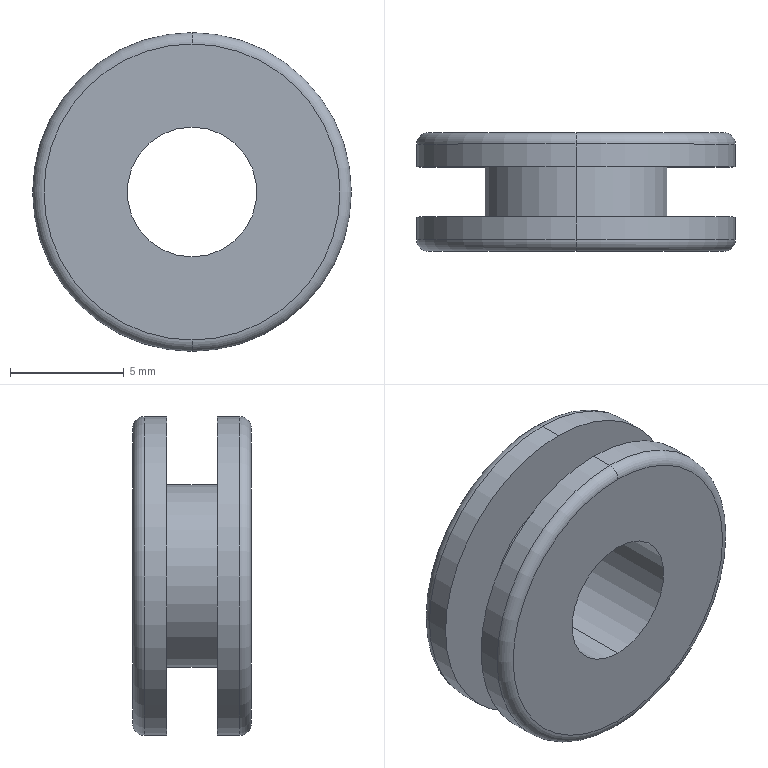Part | SolidWorks | features Revolution 1 | 1 solid | 16 faces | box 14 x 5.2 x 14 mm | volume 435.063 mm3 | cylinder 8 | torus 4 | plane 4 | commonest cylinder face diameters 14 x4 5.7 x2 8 x2
STEP:
#1=CARTESIAN_POINT('',(0.,0.5,-7.));
#2=VERTEX_POINT('',#1);
#3=CARTESIAN_POINT('',(0.,0.5,7.));
#4=VERTEX_POINT('',#3);
#5=CARTESIAN_POINT('',(0.,0.5,0.));
#6=DIRECTION('',(0.,-1.,0.));
#7=DIRECTION('',(0.,0.,-1.));
#8=AXIS2_PLACEMENT_3D('',#5,#6,#7);
#9=CIRCLE('',#8,7.);
#10=EDGE_CURVE('',#2,#4,#9,.T.);
#11=ORIENTED_EDGE('',*,*,#10,.T.);
#12=CARTESIAN_POINT('',(0.,0.,6.5));
#13=VERTEX_POINT('',#12);
#14=CARTESIAN_POINT('',(0.,0.5,6.5));
#15=DIRECTION('',(1.,0.,0.));
#16=DIRECTION('',(0.,0.,-1.));
#17=AXIS2_PLACEMENT_3D('',#14,#15,#16);
#18=CIRCLE('',#17,0.5);
#19=EDGE_CURVE('',#4,#13,#18,.T.);
#20=ORIENTED_EDGE('',*,*,#19,.T.);
#21=CARTESIAN_POINT('',(0.,0.,-6.5));
#22=VERTEX_POINT('',#21);
#23=CARTESIAN_POINT('',(0.,0.,0.));
#24=DIRECTION('',(0.,-1.,0.));
#25=DIRECTION('',(0.,0.,-1.));
#26=AXIS2_PLACEMENT_3D('',#23,#24,#25);
#27=CIRCLE('',#26,6.5);
#28=EDGE_CURVE('',#22,#13,#27,.T.);
#29=ORIENTED_EDGE('',*,*,#28,.F.);
#30=CARTESIAN_POINT('',(0.,0.5,-6.5));
#31=DIRECTION('',(-1.,0.,0.));
#32=DIRECTION('',(0.,0.,1.));
#33=AXIS2_PLACEMENT_3D('',#30,#31,#32);
#34=CIRCLE('',#33,0.5);
#35=EDGE_CURVE('',#2,#22,#34,.T.);
#36=ORIENTED_EDGE('',*,*,#35,.F.);
#37=EDGE_LOOP('',(#11,#20,#29,#36));
#38=FACE_OUTER_BOUND('',#37,.T.);
#39=CARTESIAN_POINT('',(0.,0.5,0.));
#40=DIRECTION('',(0.,-1.,0.));
#41=DIRECTION('',(0.,0.,-1.));
#42=AXIS2_PLACEMENT_3D('',#39,#40,#41);
#43=TOROIDAL_SURFACE('',#42,6.5,0.5);
#44=ADVANCED_FACE('',(#38),#43,.T.);
#45=CARTESIAN_POINT('',(0.,1.5,-7.));
#46=VERTEX_POINT('',#45);
#47=CARTESIAN_POINT('',(0.,1.5,7.));
#48=VERTEX_POINT('',#47);
#49=CARTESIAN_POINT('',(0.,1.5,0.));
#50=DIRECTION('',(0.,-1.,0.));
#51=DIRECTION('',(0.,0.,-1.));
#52=AXIS2_PLACEMENT_3D('',#49,#50,#51);
#53=CIRCLE('',#52,7.);
#54=EDGE_CURVE('',#46,#48,#53,.T.);
#55=ORIENTED_EDGE('',*,*,#54,.T.);
#56=CARTESIAN_POINT('',(0.,0.,7.));
#57=DIRECTION('',(0.,-1.,0.));
#58=VECTOR('',#57,1000.);
#59=LINE('',#56,#58);
#60=EDGE_CURVE('',#48,#4,#59,.T.);
#61=ORIENTED_EDGE('',*,*,#60,.T.);
#62=ORIENTED_EDGE('',*,*,#10,.F.);
#63=CARTESIAN_POINT('',(0.,0.,-7.));
#64=DIRECTION('',(0.,-1.,0.));
#65=VECTOR('',#64,1000.);
#66=LINE('',#63,#65);
#67=EDGE_CURVE('',#46,#2,#66,.T.);
#68=ORIENTED_EDGE('',*,*,#67,.F.);
#69=EDGE_LOOP('',(#55,#61,#62,#68));
#70=FACE_OUTER_BOUND('',#69,.T.);
#71=CARTESIAN_POINT('',(0.,0.,0.));
#72=DIRECTION('',(0.,-1.,0.));
#73=DIRECTION('',(0.,0.,-1.));
#74=AXIS2_PLACEMENT_3D('',#71,#72,#73);
#75=CYLINDRICAL_SURFACE('',#74,7.);
#76=ADVANCED_FACE('',(#70),#75,.T.);
#77=CARTESIAN_POINT('',(0.,3.7,-4.));
#78=VERTEX_POINT('',#77);
#79=CARTESIAN_POINT('',(0.,3.7,4.));
#80=VERTEX_POINT('',#79);
#81=CARTESIAN_POINT('',(0.,3.7,0.));
#82=DIRECTION('',(0.,-1.,0.));
#83=DIRECTION('',(0.,0.,-1.));
#84=AXIS2_PLACEMENT_3D('',#81,#82,#83);
#85=CIRCLE('',#84,4.);
#86=EDGE_CURVE('',#78,#80,#85,.T.);
#87=ORIENTED_EDGE('',*,*,#86,.T.);
#88=CARTESIAN_POINT('',(0.,1.5,4.));
#89=VERTEX_POINT('',#88);
#90=CARTESIAN_POINT('',(0.,0.,4.));
#91=DIRECTION('',(0.,-1.,0.));
#92=VECTOR('',#91,1000.);
#93=LINE('',#90,#92);
#94=EDGE_CURVE('',#80,#89,#93,.T.);
#95=ORIENTED_EDGE('',*,*,#94,.T.);
#96=CARTESIAN_POINT('',(0.,1.5,-4.));
#97=VERTEX_POINT('',#96);
#98=CARTESIAN_POINT('',(0.,1.5,0.));
#99=DIRECTION('',(0.,-1.,0.));
#100=DIRECTION('',(0.,0.,-1.));
#101=AXIS2_PLACEMENT_3D('',#98,#99,#100);
#102=CIRCLE('',#101,4.);
#103=EDGE_CURVE('',#97,#89,#102,.T.);
#104=ORIENTED_EDGE('',*,*,#103,.F.);
#105=CARTESIAN_POINT('',(0.,0.,-4.));
#106=DIRECTION('',(0.,-1.,0.));
#107=VECTOR('',#106,1000.);
#108=LINE('',#105,#107);
#109=EDGE_CURVE('',#78,#97,#108,.T.);
#110=ORIENTED_EDGE('',*,*,#109,.F.);
#111=EDGE_LOOP('',(#87,#95,#104,#110));
#112=FACE_OUTER_BOUND('',#111,.T.);
#113=CARTESIAN_POINT('',(0.,0.,0.));
#114=DIRECTION('',(0.,-1.,0.));
#115=DIRECTION('',(0.,0.,-1.));
#116=AXIS2_PLACEMENT_3D('',#113,#114,#115);
#117=CYLINDRICAL_SURFACE('',#116,4.);
#118=ADVANCED_FACE('',(#112),#117,.T.);
#119=CARTESIAN_POINT('',(0.,4.7,-7.));
#120=VERTEX_POINT('',#119);
#121=CARTESIAN_POINT('',(0.,4.7,7.));
#122=VERTEX_POINT('',#121);
#123=CARTESIAN_POINT('',(0.,4.7,0.));
#124=DIRECTION('',(0.,-1.,0.));
#125=DIRECTION('',(0.,0.,-1.));
#126=AXIS2_PLACEMENT_3D('',#123,#124,#125);
#127=CIRCLE('',#126,7.);
#128=EDGE_CURVE('',#120,#122,#127,.T.);
#129=ORIENTED_EDGE('',*,*,#128,.T.);
#130=CARTESIAN_POINT('',(0.,3.7,7.));
#131=VERTEX_POINT('',#130);
#132=CARTESIAN_POINT('',(0.,0.,7.));
#133=DIRECTION('',(0.,-1.,0.));
#134=VECTOR('',#133,1000.);
#135=LINE('',#132,#134);
#136=EDGE_CURVE('',#122,#131,#135,.T.);
#137=ORIENTED_EDGE('',*,*,#136,.T.);
#138=CARTESIAN_POINT('',(0.,3.7,-7.));
#139=VERTEX_POINT('',#138);
#140=CARTESIAN_POINT('',(0.,3.7,0.));
#141=DIRECTION('',(0.,-1.,0.));
#142=DIRECTION('',(0.,0.,-1.));
#143=AXIS2_PLACEMENT_3D('',#140,#141,#142);
#144=CIRCLE('',#143,7.);
#145=EDGE_CURVE('',#139,#131,#144,.T.);
#146=ORIENTED_EDGE('',*,*,#145,.F.);
#147=CARTESIAN_POINT('',(0.,0.,-7.));
#148=DIRECTION('',(0.,-1.,0.));
#149=VECTOR('',#148,1000.);
#150=LINE('',#147,#149);
#151=EDGE_CURVE('',#120,#139,#150,.T.);
#152=ORIENTED_EDGE('',*,*,#151,.F.);
#153=EDGE_LOOP('',(#129,#137,#146,#152));
#154=FACE_OUTER_BOUND('',#153,.T.);
#155=CARTESIAN_POINT('',(0.,0.,0.));
#156=DIRECTION('',(0.,-1.,0.));
#157=DIRECTION('',(0.,0.,-1.));
#158=AXIS2_PLACEMENT_3D('',#155,#156,#157);
#159=CYLINDRICAL_SURFACE('',#158,7.);
#160=ADVANCED_FACE('',(#154),#159,.T.);
#161=CARTESIAN_POINT('',(0.,5.2,-6.5));
#162=VERTEX_POINT('',#161);
#163=CARTESIAN_POINT('',(0.,5.2,6.5));
#164=VERTEX_POINT('',#163);
#165=CARTESIAN_POINT('',(0.,5.2,0.));
#166=DIRECTION('',(0.,-1.,0.));
#167=DIRECTION('',(0.,0.,-1.));
#168=AXIS2_PLACEMENT_3D('',#165,#166,#167);
#169=CIRCLE('',#168,6.5);
#170=EDGE_CURVE('',#162,#164,#169,.T.);
#171=ORIENTED_EDGE('',*,*,#170,.T.);
#172=CARTESIAN_POINT('',(0.,4.7,6.5));
#173=DIRECTION('',(1.,0.,0.));
#174=DIRECTION('',(0.,0.,-1.));
#175=AXIS2_PLACEMENT_3D('',#172,#173,#174);
#176=CIRCLE('',#175,0.5);
#177=EDGE_CURVE('',#164,#122,#176,.T.);
#178=ORIENTED_EDGE('',*,*,#177,.T.);
#179=ORIENTED_EDGE('',*,*,#128,.F.);
#180=CARTESIAN_POINT('',(0.,4.7,-6.5));
#181=DIRECTION('',(-1.,0.,0.));
#182=DIRECTION('',(0.,0.,1.));
#183=AXIS2_PLACEMENT_3D('',#180,#181,#182);
#184=CIRCLE('',#183,0.5);
#185=EDGE_CURVE('',#162,#120,#184,.T.);
#186=ORIENTED_EDGE('',*,*,#185,.F.);
#187=EDGE_LOOP('',(#171,#178,#179,#186));
#188=FACE_OUTER_BOUND('',#187,.T.);
#189=CARTESIAN_POINT('',(0.,4.7,0.));
#190=DIRECTION('',(0.,-1.,0.));
#191=DIRECTION('',(0.,0.,-1.));
#192=AXIS2_PLACEMENT_3D('',#189,#190,#191);
#193=TOROIDAL_SURFACE('',#192,6.5,0.5);
#194=ADVANCED_FACE('',(#188),#193,.T.);
#195=CARTESIAN_POINT('',(0.,5.2,2.85));
#196=VERTEX_POINT('',#195);
#197=CARTESIAN_POINT('',(0.,5.2,-2.85));
#198=VERTEX_POINT('',#197);
#199=CARTESIAN_POINT('',(0.,5.2,0.));
#200=DIRECTION('',(0.,-1.,0.));
#201=DIRECTION('',(0.,0.,-1.));
#202=AXIS2_PLACEMENT_3D('',#199,#200,#201);
#203=CIRCLE('',#202,2.85);
#204=EDGE_CURVE('',#196,#198,#203,.T.);
#205=ORIENTED_EDGE('',*,*,#204,.F.);
#206=CARTESIAN_POINT('',(0.,0.,2.85));
#207=VERTEX_POINT('',#206);
#208=CARTESIAN_POINT('',(0.,0.,2.85));
#209=DIRECTION('',(0.,-1.,0.));
#210=VECTOR('',#209,1000.);
#211=LINE('',#208,#210);
#212=EDGE_CURVE('',#196,#207,#211,.T.);
#213=ORIENTED_EDGE('',*,*,#212,.T.);
#214=CARTESIAN_POINT('',(0.,0.,-2.85));
#215=VERTEX_POINT('',#214);
#216=CARTESIAN_POINT('',(0.,0.,0.));
#217=DIRECTION('',(0.,-1.,0.));
#218=DIRECTION('',(0.,0.,-1.));
#219=AXIS2_PLACEMENT_3D('',#216,#217,#218);
#220=CIRCLE('',#219,2.85);
#221=EDGE_CURVE('',#207,#215,#220,.T.);
#222=ORIENTED_EDGE('',*,*,#221,.T.);
#223=CARTESIAN_POINT('',(0.,0.,-2.85));
#224=DIRECTION('',(0.,-1.,0.));
#225=VECTOR('',#224,1000.);
#226=LINE('',#223,#225);
#227=EDGE_CURVE('',#198,#215,#226,.T.);
#228=ORIENTED_EDGE('',*,*,#227,.F.);
#229=EDGE_LOOP('',(#205,#213,#222,#228));
#230=FACE_OUTER_BOUND('',#229,.T.);
#231=CARTESIAN_POINT('',(0.,0.,0.));
#232=DIRECTION('',(0.,-1.,0.));
#233=DIRECTION('',(0.,0.,-1.));
#234=AXIS2_PLACEMENT_3D('',#231,#232,#233);
#235=CYLINDRICAL_SURFACE('',#234,2.85);
#236=ADVANCED_FACE('',(#230),#235,.F.);
#237=ORIENTED_EDGE('',*,*,#212,.F.);
#238=CARTESIAN_POINT('',(0.,5.2,0.));
#239=DIRECTION('',(0.,-1.,0.));
#240=DIRECTION('',(0.,0.,-1.));
#241=AXIS2_PLACEMENT_3D('',#238,#239,#240);
#242=CIRCLE('',#241,2.85);
#243=EDGE_CURVE('',#198,#196,#242,.T.);
#244=ORIENTED_EDGE('',*,*,#243,.F.);
#245=ORIENTED_EDGE('',*,*,#227,.T.);
#246=CARTESIAN_POINT('',(0.,0.,0.));
#247=DIRECTION('',(0.,-1.,0.));
#248=DIRECTION('',(0.,0.,-1.));
#249=AXIS2_PLACEMENT_3D('',#246,#247,#248);
#250=CIRCLE('',#249,2.85);
#251=EDGE_CURVE('',#215,#207,#250,.T.);
#252=ORIENTED_EDGE('',*,*,#251,.T.);
#253=EDGE_LOOP('',(#237,#244,#245,#252));
#254=FACE_OUTER_BOUND('',#253,.T.);
#255=CARTESIAN_POINT('',(0.,0.,0.));
#256=DIRECTION('',(0.,-1.,0.));
#257=DIRECTION('',(0.,0.,-1.));
#258=AXIS2_PLACEMENT_3D('',#255,#256,#257);
#259=CYLINDRICAL_SURFACE('',#258,2.85);
#260=ADVANCED_FACE('',(#254),#259,.F.);
#261=ORIENTED_EDGE('',*,*,#243,.T.);
#262=ORIENTED_EDGE('',*,*,#204,.T.);
#263=EDGE_LOOP('',(#261,#262));
#264=FACE_BOUND('',#263,.T.);
#265=ORIENTED_EDGE('',*,*,#170,.F.);
#266=CARTESIAN_POINT('',(0.,5.2,0.));
#267=DIRECTION('',(0.,-1.,0.));
#268=DIRECTION('',(0.,0.,-1.));
#269=AXIS2_PLACEMENT_3D('',#266,#267,#268);
#270=CIRCLE('',#269,6.5);
#271=EDGE_CURVE('',#164,#162,#270,.T.);
#272=ORIENTED_EDGE('',*,*,#271,.F.);
#273=EDGE_LOOP('',(#265,#272));
#274=FACE_OUTER_BOUND('',#273,.T.);
#275=CARTESIAN_POINT('',(2.85,5.2,0.));
#276=DIRECTION('',(0.,1.,0.));
#277=DIRECTION('',(0.,0.,1.));
#278=AXIS2_PLACEMENT_3D('',#275,#276,#277);
#279=PLANE('',#278);
#280=ADVANCED_FACE('',(#264,#274),#279,.T.);
#281=ORIENTED_EDGE('',*,*,#177,.F.);
#282=ORIENTED_EDGE('',*,*,#271,.T.);
#283=ORIENTED_EDGE('',*,*,#185,.T.);
#284=CARTESIAN_POINT('',(0.,4.7,0.));
#285=DIRECTION('',(0.,-1.,0.));
#286=DIRECTION('',(0.,0.,-1.));
#287=AXIS2_PLACEMENT_3D('',#284,#285,#286);
#288=CIRCLE('',#287,7.);
#289=EDGE_CURVE('',#122,#120,#288,.T.);
#290=ORIENTED_EDGE('',*,*,#289,.F.);
#291=EDGE_LOOP('',(#281,#282,#283,#290));
#292=FACE_OUTER_BOUND('',#291,.T.);
#293=CARTESIAN_POINT('',(0.,4.7,0.));
#294=DIRECTION('',(0.,-1.,0.));
#295=DIRECTION('',(0.,0.,-1.));
#296=AXIS2_PLACEMENT_3D('',#293,#294,#295);
#297=TOROIDAL_SURFACE('',#296,6.5,0.5);
#298=ADVANCED_FACE('',(#292),#297,.T.);
#299=ORIENTED_EDGE('',*,*,#136,.F.);
#300=ORIENTED_EDGE('',*,*,#289,.T.);
#301=ORIENTED_EDGE('',*,*,#151,.T.);
#302=CARTESIAN_POINT('',(0.,3.7,0.));
#303=DIRECTION('',(0.,-1.,0.));
#304=DIRECTION('',(0.,0.,-1.));
#305=AXIS2_PLACEMENT_3D('',#302,#303,#304);
#306=CIRCLE('',#305,7.);
#307=EDGE_CURVE('',#131,#139,#306,.T.);
#308=ORIENTED_EDGE('',*,*,#307,.F.);
#309=EDGE_LOOP('',(#299,#300,#301,#308));
#310=FACE_OUTER_BOUND('',#309,.T.);
#311=CARTESIAN_POINT('',(0.,0.,0.));
#312=DIRECTION('',(0.,-1.,0.));
#313=DIRECTION('',(0.,0.,-1.));
#314=AXIS2_PLACEMENT_3D('',#311,#312,#313);
#315=CYLINDRICAL_SURFACE('',#314,7.);
#316=ADVANCED_FACE('',(#310),#315,.T.);
#317=ORIENTED_EDGE('',*,*,#145,.T.);
#318=ORIENTED_EDGE('',*,*,#307,.T.);
#319=EDGE_LOOP('',(#317,#318));
#320=FACE_OUTER_BOUND('',#319,.T.);
#321=ORIENTED_EDGE('',*,*,#86,.F.);
#322=CARTESIAN_POINT('',(0.,3.7,0.));
#323=DIRECTION('',(0.,-1.,0.));
#324=DIRECTION('',(0.,0.,-1.));
#325=AXIS2_PLACEMENT_3D('',#322,#323,#324);
#326=CIRCLE('',#325,4.);
#327=EDGE_CURVE('',#80,#78,#326,.T.);
#328=ORIENTED_EDGE('',*,*,#327,.F.);
#329=EDGE_LOOP('',(#321,#328));
#330=FACE_BOUND('',#329,.T.);
#331=CARTESIAN_POINT('',(7.,3.7,0.));
#332=DIRECTION('',(0.,-1.,0.));
#333=DIRECTION('',(0.,0.,-1.));
#334=AXIS2_PLACEMENT_3D('',#331,#332,#333);
#335=PLANE('',#334);
#336=ADVANCED_FACE('',(#320,#330),#335,.T.);
#337=ORIENTED_EDGE('',*,*,#94,.F.);
#338=ORIENTED_EDGE('',*,*,#327,.T.);
#339=ORIENTED_EDGE('',*,*,#109,.T.);
#340=CARTESIAN_POINT('',(0.,1.5,0.));
#341=DIRECTION('',(0.,-1.,0.));
#342=DIRECTION('',(0.,0.,-1.));
#343=AXIS2_PLACEMENT_3D('',#340,#341,#342);
#344=CIRCLE('',#343,4.);
#345=EDGE_CURVE('',#89,#97,#344,.T.);
#346=ORIENTED_EDGE('',*,*,#345,.F.);
#347=EDGE_LOOP('',(#337,#338,#339,#346));
#348=FACE_OUTER_BOUND('',#347,.T.);
#349=CARTESIAN_POINT('',(0.,0.,0.));
#350=DIRECTION('',(0.,-1.,0.));
#351=DIRECTION('',(0.,0.,-1.));
#352=AXIS2_PLACEMENT_3D('',#349,#350,#351);
#353=CYLINDRICAL_SURFACE('',#352,4.);
#354=ADVANCED_FACE('',(#348),#353,.T.);
#355=ORIENTED_EDGE('',*,*,#103,.T.);
#356=ORIENTED_EDGE('',*,*,#345,.T.);
#357=EDGE_LOOP('',(#355,#356));
#358=FACE_BOUND('',#357,.T.);
#359=ORIENTED_EDGE('',*,*,#54,.F.);
#360=CARTESIAN_POINT('',(0.,1.5,0.));
#361=DIRECTION('',(0.,-1.,0.));
#362=DIRECTION('',(0.,0.,-1.));
#363=AXIS2_PLACEMENT_3D('',#360,#361,#362);
#364=CIRCLE('',#363,7.);
#365=EDGE_CURVE('',#48,#46,#364,.T.);
#366=ORIENTED_EDGE('',*,*,#365,.F.);
#367=EDGE_LOOP('',(#359,#366));
#368=FACE_OUTER_BOUND('',#367,.T.);
#369=CARTESIAN_POINT('',(4.,1.5,0.));
#370=DIRECTION('',(0.,1.,0.));
#371=DIRECTION('',(0.,0.,1.));
#372=AXIS2_PLACEMENT_3D('',#369,#370,#371);
#373=PLANE('',#372);
#374=ADVANCED_FACE('',(#358,#368),#373,.T.);
#375=ORIENTED_EDGE('',*,*,#60,.F.);
#376=ORIENTED_EDGE('',*,*,#365,.T.);
#377=ORIENTED_EDGE('',*,*,#67,.T.);
#378=CARTESIAN_POINT('',(0.,0.5,0.));
#379=DIRECTION('',(0.,-1.,0.));
#380=DIRECTION('',(0.,0.,-1.));
#381=AXIS2_PLACEMENT_3D('',#378,#379,#380);
#382=CIRCLE('',#381,7.);
#383=EDGE_CURVE('',#4,#2,#382,.T.);
#384=ORIENTED_EDGE('',*,*,#383,.F.);
#385=EDGE_LOOP('',(#375,#376,#377,#384));
#386=FACE_OUTER_BOUND('',#385,.T.);
#387=CARTESIAN_POINT('',(0.,0.,0.));
#388=DIRECTION('',(0.,-1.,0.));
#389=DIRECTION('',(0.,0.,-1.));
#390=AXIS2_PLACEMENT_3D('',#387,#388,#389);
#391=CYLINDRICAL_SURFACE('',#390,7.);
#392=ADVANCED_FACE('',(#386),#391,.T.);
#393=ORIENTED_EDGE('',*,*,#19,.F.);
#394=ORIENTED_EDGE('',*,*,#383,.T.);
#395=ORIENTED_EDGE('',*,*,#35,.T.);
#396=CARTESIAN_POINT('',(0.,0.,0.));
#397=DIRECTION('',(0.,-1.,0.));
#398=DIRECTION('',(0.,0.,-1.));
#399=AXIS2_PLACEMENT_3D('',#396,#397,#398);
#400=CIRCLE('',#399,6.5);
#401=EDGE_CURVE('',#13,#22,#400,.T.);
#402=ORIENTED_EDGE('',*,*,#401,.F.);
#403=EDGE_LOOP('',(#393,#394,#395,#402));
#404=FACE_OUTER_BOUND('',#403,.T.);
#405=CARTESIAN_POINT('',(0.,0.5,0.));
#406=DIRECTION('',(0.,-1.,0.));
#407=DIRECTION('',(0.,0.,-1.));
#408=AXIS2_PLACEMENT_3D('',#405,#406,#407);
#409=TOROIDAL_SURFACE('',#408,6.5,0.5);
#410=ADVANCED_FACE('',(#404),#409,.T.);
#411=ORIENTED_EDGE('',*,*,#28,.T.);
#412=ORIENTED_EDGE('',*,*,#401,.T.);
#413=EDGE_LOOP('',(#411,#412));
#414=FACE_OUTER_BOUND('',#413,.T.);
#415=ORIENTED_EDGE('',*,*,#251,.F.);
#416=ORIENTED_EDGE('',*,*,#221,.F.);
#417=EDGE_LOOP('',(#415,#416));
#418=FACE_BOUND('',#417,.T.);
#419=CARTESIAN_POINT('',(6.5,0.,0.));
#420=DIRECTION('',(0.,-1.,0.));
#421=DIRECTION('',(0.,0.,-1.));
#422=AXIS2_PLACEMENT_3D('',#419,#420,#421);
#423=PLANE('',#422);
#424=ADVANCED_FACE('',(#414,#418),#423,.T.);
#425=CLOSED_SHELL('',(#44,#76,#118,#160,#194,#236,#260,#280,#298,#316,#336,#354,#374,#392,#410,#424));
#426=MANIFOLD_SOLID_BREP('',#425);
#427=CARTESIAN_POINT('',(0.,0.,0.));
#428=DIRECTION('',(0.,0.,1.));
#429=DIRECTION('',(1.,0.,0.));
#430=AXIS2_PLACEMENT_3D('',#427,#428,#429);
#431=(LENGTH_UNIT()NAMED_UNIT(*)SI_UNIT(.MILLI.,.METRE.));
#432=UNCERTAINTY_MEASURE_WITH_UNIT(LENGTH_MEASURE(0.00001),#431,'','');
#433=(NAMED_UNIT(*)PLANE_ANGLE_UNIT()SI_UNIT($,.RADIAN.));
#434=(NAMED_UNIT(*)SI_UNIT($,.STERADIAN.)SOLID_ANGLE_UNIT());
#435=(GEOMETRIC_REPRESENTATION_CONTEXT(3)GLOBAL_UNCERTAINTY_ASSIGNED_CONTEXT((#432))GLOBAL_UNIT_ASSIGNED_CONTEXT((#431,#433,#434))REPRESENTATION_CONTEXT('',''));
#436=ADVANCED_BREP_SHAPE_REPRESENTATION('',(#426,#430),#435);